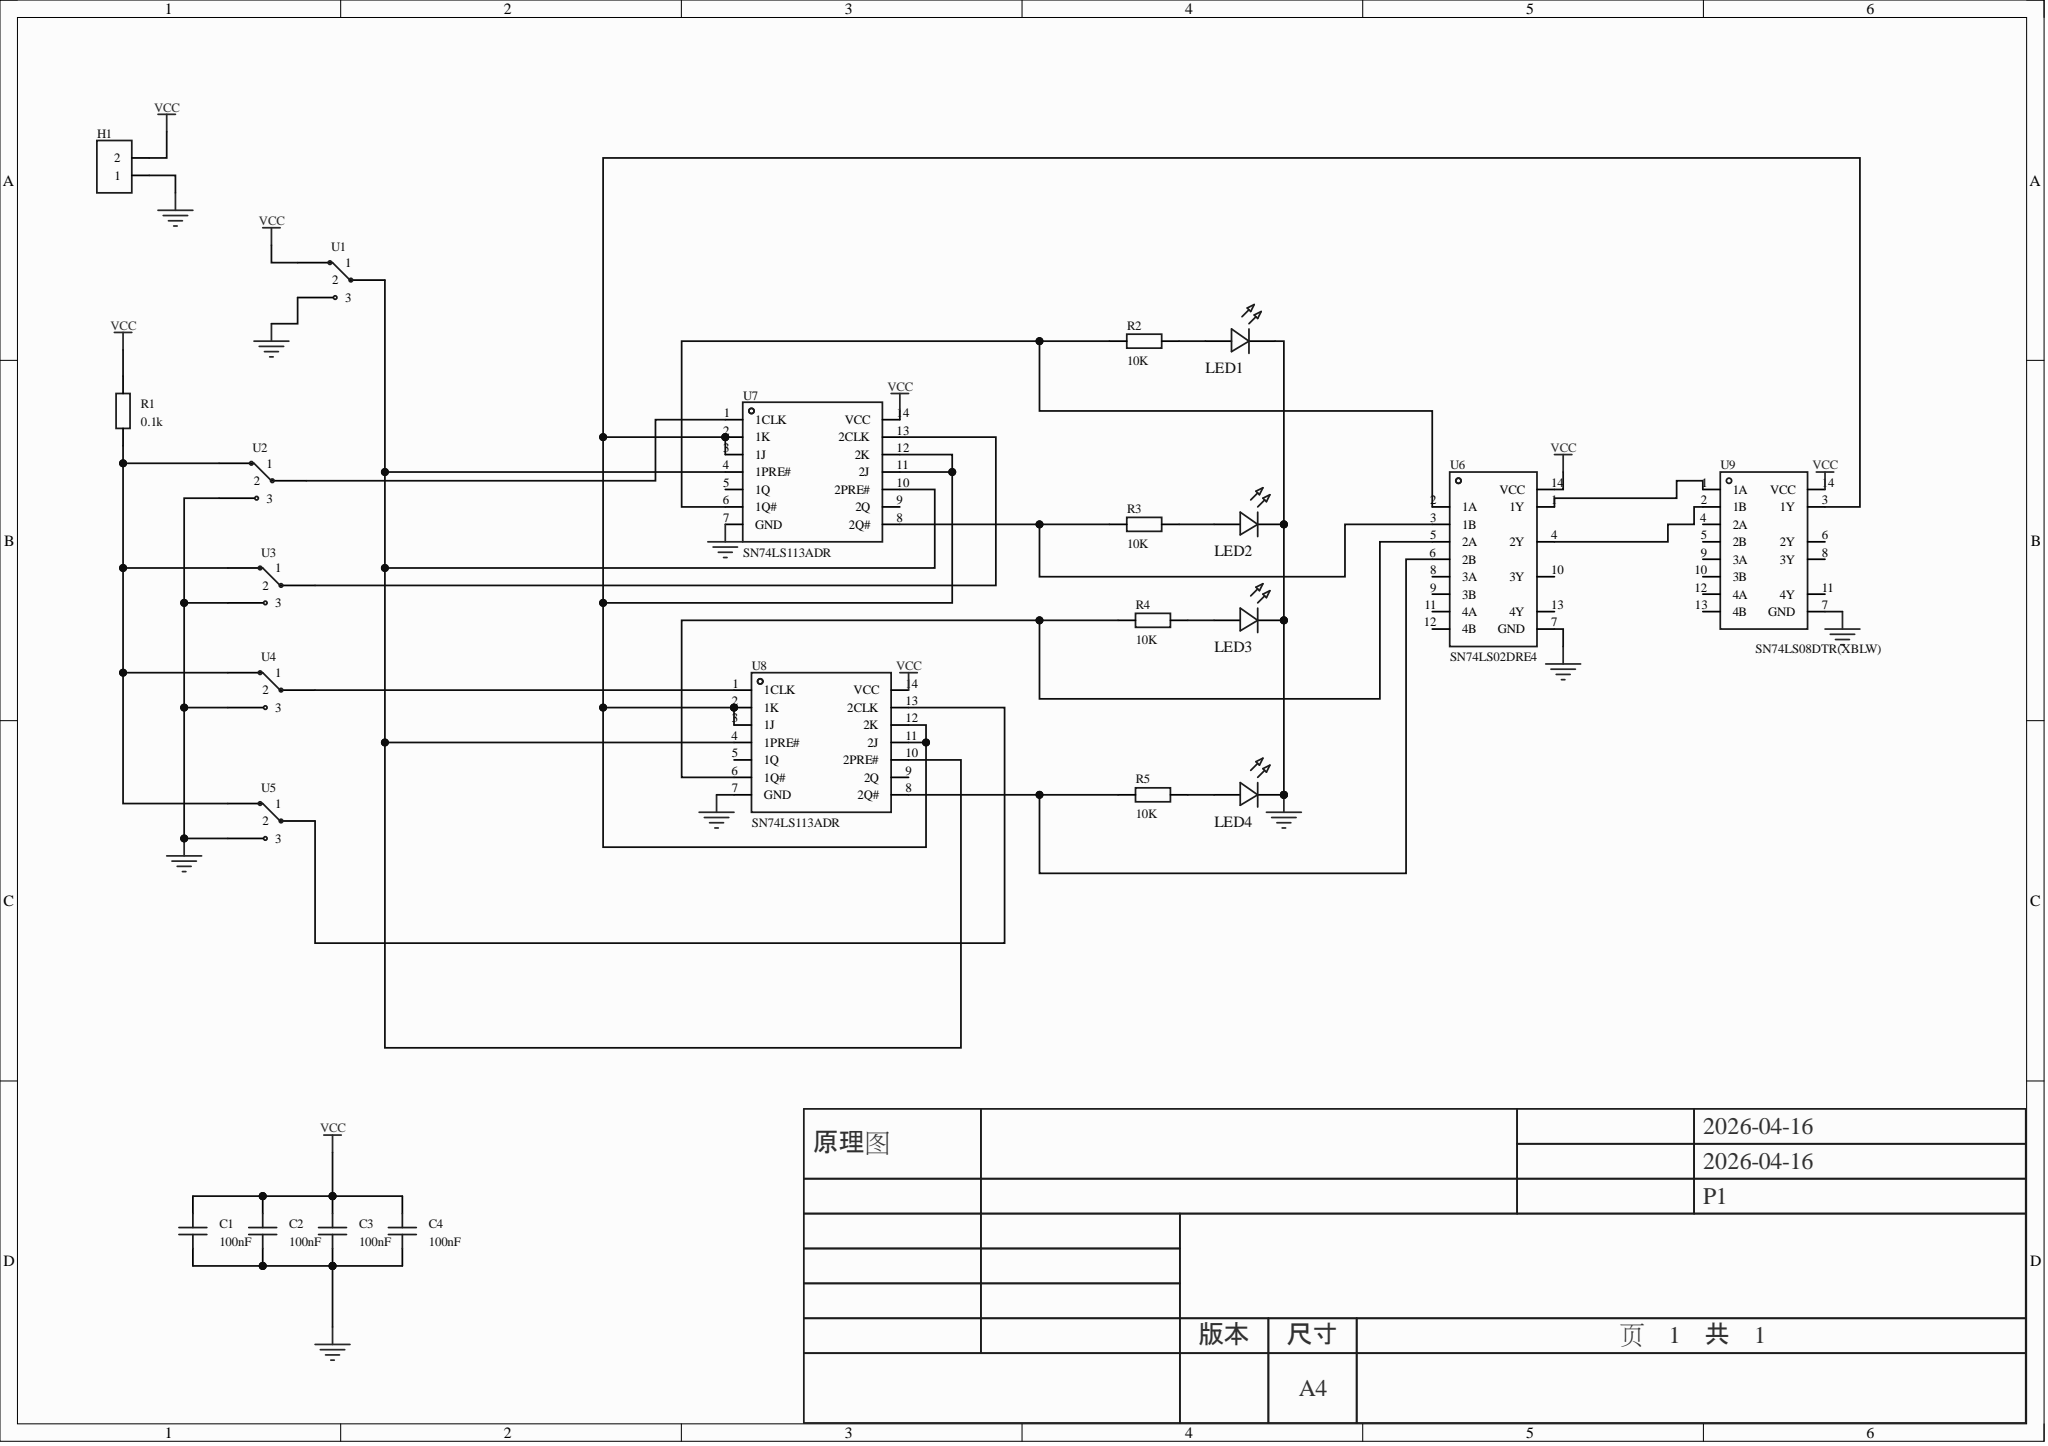Circuit board | Altium Designer | 23 parts | 19 nets
Bill of materials:
Comment,Description,Designator,Footprint,LibRef,Quantity
"100nF","","C1, C2, C3, C4","C0603","CAP_0603","4"
"","","H1","HDR-TH_2P-P2.54-V-F","HDR-F_2.54_1x2P","1"
"","","LED1, LED2, LED3, LED4","LED_0603","LED_0603-R","4"
"0.1k","","R1","R0603","Res_0603","1"
"10K","","R2, R3, R4, R5","R0603","Res_0603","4"
"","","U1, U2, U3, U4, U5","单刀双掷","单刀双掷开关","5"
"SN74LS02DRE4","逻辑类型:或非门;通道数:4;工作电压:4.75V~5.25V;传播延迟(tpd):15ns@5V,15pF;","U6","SOIC-14_L8.7-W3.9-P1.27-LS6.0-BL","SN74LS02DRE4","1"
"SN74LS113ADR","","U7, U8","SOIC-14_L8.6-W3.9-P1.27-LS6.0-BL","SN74LS113ADR","2"
"SN74LS08DTR(XBLW)","","U9","SOIC-14_L8.7-W3.9-P1.27-LS6.0-BL","SN74LS08DTR(XBLW)","1"
Netlist (Protel format):
[
C1
C0603
100nF



]
[
C2
C0603
100nF



]
[
C3
C0603
100nF



]
[
C4
C0603
100nF



]
[
H1
HDR-TH_2P-P2.54-V-F




]
[
LED1
LED_0603




]
[
LED2
LED_0603




]
[
LED3
LED_0603




]
[
LED4
LED_0603




]
[
R1
R0603
0.1k



]
[
R2
R0603
10K



]
[
R3
R0603
10K



]
[
R4
R0603
10K



]
[
R5
R0603
10K



]
[
U1
单刀双掷




]
[
U2
单刀双掷




]
[
U3
单刀双掷




]
[
U4
单刀双掷




]
[
U5
单刀双掷




]
[
U6
SOIC-14_L8.7-W3.9-P1.27-LS6.0-BL
SN74LS02DRE4



]
[
U7
SOIC-14_L8.6-W3.9-P1.27-LS6.0-BL
SN74LS113ADR



]
[
U8
SOIC-14_L8.6-W3.9-P1.27-LS6.0-BL
SN74LS113ADR



]
[
U9
SOIC-14_L8.7-W3.9-P1.27-LS6.0-BL
SN74LS08DTR(XBLW)



]
(
VCC
C1-2
C2-2
C3-2
C4-2
H1-2
R1-2
U1-1
U6-14
U7-14
U8-14
U9-14
)
(
NetU7_2
U7-2
U7-3
U7-11
U7-12
U8-2
U8-3
U8-11
U8-12
U9-3
)
(
NetU6_4
U6-4
U9-2
)
(
NetU6_1
U6-1
U9-1
)
(
NetU5_2
U5-2
U8-13
)
(
NetU4_2
U4-2
U8-1
)
(
NetU3_2
U3-2
U7-13
)
(
NetU2_2
U2-2
U7-1
)
(
NetU1_2
U1-2
U7-4
U7-10
U8-4
U8-10
)
(
NetR5_1
R5-1
U6-6
U8-8
)
(
NetR4_1
R4-1
U6-5
U8-6
)
(
NetR3_1
R3-1
U6-3
U7-8
)
(
NetR2_1
R2-1
U6-2
U7-6
)
(
NetR1_1
R1-1
U2-1
U3-1
U4-1
U5-1
)
(
NetLED4_2
LED4-2
R5-2
)
(
NetLED3_2
LED3-2
R4-2
)
(
NetLED2_2
LED2-2
R3-2
)
(
NetLED1_2
LED1-2
R2-2
)
(
GND
C1-1
C2-1
C3-1
C4-1
H1-1
LED1-1
LED2-1
LED3-1
LED4-1
U1-3
U2-3
U3-3
U4-3
U5-3
U6-7
U7-7
U8-7
U9-7
)